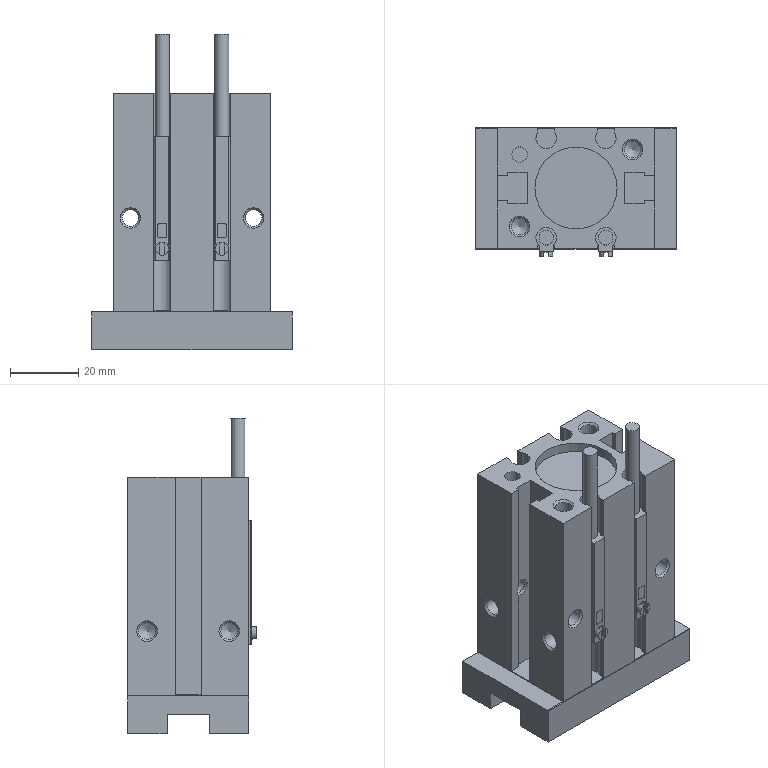Part | NX | features WGY01-16-6-2-002 2 | 1 solid | 148 faces | box 58.5 x 37.65 x 92.25 mm | volume 104769 mm3 | plane 92 | cylinder 42 | cone 14 | commonest cylinder face diameters 1.2 x8 4.863 x8 6.03 x6 0.3 x4 5.1 x4 6.045 x4